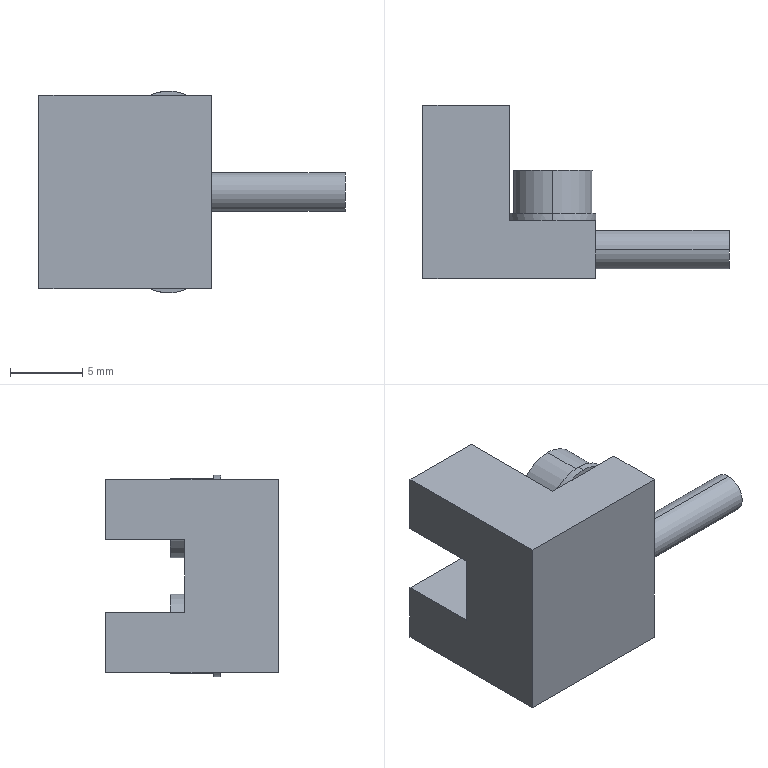Part | STEP file | QA-EE_SX91_R1M_lx | 1 solid | 33 faces | box 21.25 x 12 x 14 mm | volume 1345 mm3 | plane 23 | cylinder 10 | commonest cylinder face diameters 5.5 x4 6 x4 2.7 x2